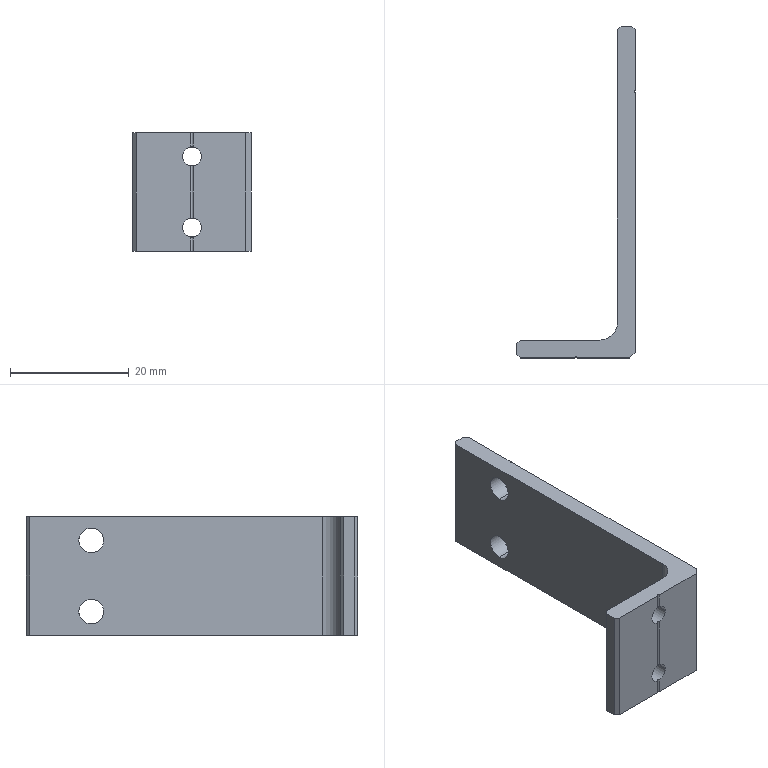Part | SolidWorks | features BaseBody 1 | 1 solid | 30 faces | box 20 x 56 x 20 mm | volume 4261 mm3 | cylinder 15 | plane 15 | commonest cylinder face diameters 0.4 x6 3.2 x4 4.2 x4 6 x1
STEP:
#1=CARTESIAN_POINT('',(20.,44.8,1.91));
#2=VERTEX_POINT('',#1);
#3=CARTESIAN_POINT('',(19.8,45.,1.9));
#4=VERTEX_POINT('',#3);
#5=CARTESIAN_POINT('',(20.,44.8,1.91));
#6=CARTESIAN_POINT('',(19.947,44.8,1.91));
#7=CARTESIAN_POINT('',(19.895,44.822,1.907));
#8=CARTESIAN_POINT('',(19.822,44.895,1.902));
#9=CARTESIAN_POINT('',(19.8,44.947,1.9));
#10=CARTESIAN_POINT('',(19.8,45.,1.9));
#11=B_SPLINE_CURVE_WITH_KNOTS('',3,(#5,#6,#7,#8,#9,#10),.UNSPECIFIED.,.F.,.F.,(4,2,4),(-0.0003126,-0.0001563,0.),.UNSPECIFIED.);
#12=EDGE_CURVE('',#2,#4,#11,.T.);
#13=ORIENTED_EDGE('',*,*,#12,.T.);
#14=CARTESIAN_POINT('',(17.,45.,1.9));
#15=VERTEX_POINT('',#14);
#16=CARTESIAN_POINT('',(37.,45.,1.9));
#17=DIRECTION('',(-1.,0.,0.));
#18=VECTOR('',#17,1000.);
#19=LINE('',#16,#18);
#20=EDGE_CURVE('',#4,#15,#19,.T.);
#21=ORIENTED_EDGE('',*,*,#20,.T.);
#22=CARTESIAN_POINT('',(17.,45.,6.1));
#23=VERTEX_POINT('',#22);
#24=CARTESIAN_POINT('',(17.,45.,4.));
#25=DIRECTION('',(-1.,0.,0.));
#26=DIRECTION('',(0.,0.,1.));
#27=AXIS2_PLACEMENT_3D('',#24,#25,#26);
#28=CIRCLE('',#27,2.1);
#29=EDGE_CURVE('',#15,#23,#28,.T.);
#30=ORIENTED_EDGE('',*,*,#29,.T.);
#31=CARTESIAN_POINT('',(19.8,45.,6.1));
#32=VERTEX_POINT('',#31);
#33=CARTESIAN_POINT('',(37.,45.,6.1));
#34=DIRECTION('',(-1.,0.,0.));
#35=VECTOR('',#34,1000.);
#36=LINE('',#33,#35);
#37=EDGE_CURVE('',#32,#23,#36,.T.);
#38=ORIENTED_EDGE('',*,*,#37,.F.);
#39=CARTESIAN_POINT('',(20.,44.8,6.09));
#40=VERTEX_POINT('',#39);
#41=CARTESIAN_POINT('',(19.8,45.,6.1));
#42=CARTESIAN_POINT('',(19.8,44.947,6.1));
#43=CARTESIAN_POINT('',(19.822,44.895,6.098));
#44=CARTESIAN_POINT('',(19.895,44.822,6.093));
#45=CARTESIAN_POINT('',(19.947,44.8,6.09));
#46=CARTESIAN_POINT('',(20.,44.8,6.09));
#47=B_SPLINE_CURVE_WITH_KNOTS('',3,(#41,#42,#43,#44,#45,#46),.UNSPECIFIED.,.F.,.F.,(4,2,4),(0.,0.0001563,0.0003126),.UNSPECIFIED.);
#48=EDGE_CURVE('',#32,#40,#47,.T.);
#49=ORIENTED_EDGE('',*,*,#48,.T.);
#50=CARTESIAN_POINT('',(20.,45.,4.));
#51=DIRECTION('',(-1.,0.,0.));
#52=DIRECTION('',(0.,0.,1.));
#53=AXIS2_PLACEMENT_3D('',#50,#51,#52);
#54=CIRCLE('',#53,2.1);
#55=EDGE_CURVE('',#2,#40,#54,.T.);
#56=ORIENTED_EDGE('',*,*,#55,.F.);
#57=EDGE_LOOP('',(#13,#21,#30,#38,#49,#56));
#58=FACE_OUTER_BOUND('',#57,.T.);
#59=CARTESIAN_POINT('',(37.,45.,4.));
#60=DIRECTION('',(-1.,0.,0.));
#61=DIRECTION('',(0.,0.,1.));
#62=AXIS2_PLACEMENT_3D('',#59,#60,#61);
#63=CYLINDRICAL_SURFACE('',#62,2.1);
#64=ADVANCED_FACE('',(#58),#63,.F.);
#65=CARTESIAN_POINT('',(20.,44.8,13.91));
#66=VERTEX_POINT('',#65);
#67=CARTESIAN_POINT('',(19.8,45.,13.9));
#68=VERTEX_POINT('',#67);
#69=CARTESIAN_POINT('',(20.,44.8,13.91));
#70=CARTESIAN_POINT('',(19.947,44.8,13.91));
#71=CARTESIAN_POINT('',(19.895,44.822,13.907));
#72=CARTESIAN_POINT('',(19.822,44.895,13.902));
#73=CARTESIAN_POINT('',(19.8,44.947,13.9));
#74=CARTESIAN_POINT('',(19.8,45.,13.9));
#75=B_SPLINE_CURVE_WITH_KNOTS('',3,(#69,#70,#71,#72,#73,#74),.UNSPECIFIED.,.F.,.F.,(4,2,4),(-0.0003126,-0.0001563,0.),.UNSPECIFIED.);
#76=EDGE_CURVE('',#66,#68,#75,.T.);
#77=ORIENTED_EDGE('',*,*,#76,.T.);
#78=CARTESIAN_POINT('',(17.,45.,13.9));
#79=VERTEX_POINT('',#78);
#80=CARTESIAN_POINT('',(37.,45.,13.9));
#81=DIRECTION('',(-1.,0.,0.));
#82=VECTOR('',#81,1000.);
#83=LINE('',#80,#82);
#84=EDGE_CURVE('',#68,#79,#83,.T.);
#85=ORIENTED_EDGE('',*,*,#84,.T.);
#86=CARTESIAN_POINT('',(17.,45.,18.1));
#87=VERTEX_POINT('',#86);
#88=CARTESIAN_POINT('',(17.,45.,16.));
#89=DIRECTION('',(-1.,0.,0.));
#90=DIRECTION('',(0.,0.,1.));
#91=AXIS2_PLACEMENT_3D('',#88,#89,#90);
#92=CIRCLE('',#91,2.1);
#93=EDGE_CURVE('',#79,#87,#92,.T.);
#94=ORIENTED_EDGE('',*,*,#93,.T.);
#95=CARTESIAN_POINT('',(19.8,45.,18.1));
#96=VERTEX_POINT('',#95);
#97=CARTESIAN_POINT('',(37.,45.,18.1));
#98=DIRECTION('',(-1.,0.,0.));
#99=VECTOR('',#98,1000.);
#100=LINE('',#97,#99);
#101=EDGE_CURVE('',#96,#87,#100,.T.);
#102=ORIENTED_EDGE('',*,*,#101,.F.);
#103=CARTESIAN_POINT('',(20.,44.8,18.09));
#104=VERTEX_POINT('',#103);
#105=CARTESIAN_POINT('',(19.8,45.,18.1));
#106=CARTESIAN_POINT('',(19.8,44.947,18.1));
#107=CARTESIAN_POINT('',(19.822,44.895,18.098));
#108=CARTESIAN_POINT('',(19.895,44.822,18.093));
#109=CARTESIAN_POINT('',(19.947,44.8,18.09));
#110=CARTESIAN_POINT('',(20.,44.8,18.09));
#111=B_SPLINE_CURVE_WITH_KNOTS('',3,(#105,#106,#107,#108,#109,#110),.UNSPECIFIED.,.F.,.F.,(4,2,4),(0.0003126,0.0004689,0.0006252),.UNSPECIFIED.);
#112=EDGE_CURVE('',#96,#104,#111,.T.);
#113=ORIENTED_EDGE('',*,*,#112,.T.);
#114=CARTESIAN_POINT('',(20.,45.,16.));
#115=DIRECTION('',(-1.,0.,0.));
#116=DIRECTION('',(0.,0.,1.));
#117=AXIS2_PLACEMENT_3D('',#114,#115,#116);
#118=CIRCLE('',#117,2.1);
#119=EDGE_CURVE('',#66,#104,#118,.T.);
#120=ORIENTED_EDGE('',*,*,#119,.F.);
#121=EDGE_LOOP('',(#77,#85,#94,#102,#113,#120));
#122=FACE_OUTER_BOUND('',#121,.T.);
#123=CARTESIAN_POINT('',(37.,45.,16.));
#124=DIRECTION('',(-1.,0.,0.));
#125=DIRECTION('',(0.,0.,1.));
#126=AXIS2_PLACEMENT_3D('',#123,#124,#125);
#127=CYLINDRICAL_SURFACE('',#126,2.1);
#128=ADVANCED_FACE('',(#122),#127,.F.);
#129=CARTESIAN_POINT('',(10.2,0.,2.413));
#130=VERTEX_POINT('',#129);
#131=CARTESIAN_POINT('',(11.6,0.,4.));
#132=VERTEX_POINT('',#131);
#133=CARTESIAN_POINT('',(10.,0.,4.));
#134=DIRECTION('',(0.,-1.,0.));
#135=DIRECTION('',(-1.,0.,0.));
#136=AXIS2_PLACEMENT_3D('',#133,#134,#135);
#137=CIRCLE('',#136,1.6);
#138=EDGE_CURVE('',#130,#132,#137,.T.);
#139=ORIENTED_EDGE('',*,*,#138,.T.);
#140=CARTESIAN_POINT('',(11.6,3.,4.));
#141=VERTEX_POINT('',#140);
#142=CARTESIAN_POINT('',(11.6,-17.,4.));
#143=DIRECTION('',(0.,1.,0.));
#144=VECTOR('',#143,1000.);
#145=LINE('',#142,#144);
#146=EDGE_CURVE('',#132,#141,#145,.T.);
#147=ORIENTED_EDGE('',*,*,#146,.T.);
#148=CARTESIAN_POINT('',(8.4,3.,4.));
#149=VERTEX_POINT('',#148);
#150=CARTESIAN_POINT('',(10.,3.,4.));
#151=DIRECTION('',(0.,1.,0.));
#152=DIRECTION('',(-1.,0.,0.));
#153=AXIS2_PLACEMENT_3D('',#150,#151,#152);
#154=CIRCLE('',#153,1.6);
#155=EDGE_CURVE('',#141,#149,#154,.T.);
#156=ORIENTED_EDGE('',*,*,#155,.T.);
#157=CARTESIAN_POINT('',(8.4,0.,4.));
#158=VERTEX_POINT('',#157);
#159=CARTESIAN_POINT('',(8.4,-17.,4.));
#160=DIRECTION('',(0.,1.,0.));
#161=VECTOR('',#160,1000.);
#162=LINE('',#159,#161);
#163=EDGE_CURVE('',#158,#149,#162,.T.);
#164=ORIENTED_EDGE('',*,*,#163,.F.);
#165=CARTESIAN_POINT('',(9.8,0.,2.413));
#166=VERTEX_POINT('',#165);
#167=CARTESIAN_POINT('',(10.,0.,4.));
#168=DIRECTION('',(0.,-1.,0.));
#169=DIRECTION('',(-1.,0.,0.));
#170=AXIS2_PLACEMENT_3D('',#167,#168,#169);
#171=CIRCLE('',#170,1.6);
#172=EDGE_CURVE('',#158,#166,#171,.T.);
#173=ORIENTED_EDGE('',*,*,#172,.T.);
#174=CARTESIAN_POINT('',(9.8,0.,2.413));
#175=CARTESIAN_POINT('',(9.8,0.0529,2.413));
#176=CARTESIAN_POINT('',(9.822,0.1046,2.41));
#177=CARTESIAN_POINT('',(9.895,0.1783,2.403));
#178=CARTESIAN_POINT('',(9.948,0.2,2.4));
#179=CARTESIAN_POINT('',(10.052,0.2,2.4));
#180=CARTESIAN_POINT('',(10.104,0.1788,2.403));
#181=CARTESIAN_POINT('',(10.179,0.1042,2.41));
#182=CARTESIAN_POINT('',(10.2,0.0529,2.413));
#183=CARTESIAN_POINT('',(10.2,0.,2.413));
#184=B_SPLINE_CURVE_WITH_KNOTS('',3,(#174,#175,#176,#177,#178,#179,#180,#181,#182,#183),.UNSPECIFIED.,.F.,.F.,(4,2,2,2,4),(0.,0.0001564,0.0003129,0.0004693,0.0006258),.UNSPECIFIED.);
#185=EDGE_CURVE('',#166,#130,#184,.T.);
#186=ORIENTED_EDGE('',*,*,#185,.T.);
#187=EDGE_LOOP('',(#139,#147,#156,#164,#173,#186));
#188=FACE_OUTER_BOUND('',#187,.T.);
#189=CARTESIAN_POINT('',(10.,-17.,4.));
#190=DIRECTION('',(0.,1.,0.));
#191=DIRECTION('',(-1.,0.,0.));
#192=AXIS2_PLACEMENT_3D('',#189,#190,#191);
#193=CYLINDRICAL_SURFACE('',#192,1.6);
#194=ADVANCED_FACE('',(#188),#193,.F.);
#195=CARTESIAN_POINT('',(10.2,0.,14.413));
#196=VERTEX_POINT('',#195);
#197=CARTESIAN_POINT('',(11.6,0.,16.));
#198=VERTEX_POINT('',#197);
#199=CARTESIAN_POINT('',(10.,0.,16.));
#200=DIRECTION('',(0.,-1.,0.));
#201=DIRECTION('',(-1.,0.,0.));
#202=AXIS2_PLACEMENT_3D('',#199,#200,#201);
#203=CIRCLE('',#202,1.6);
#204=EDGE_CURVE('',#196,#198,#203,.T.);
#205=ORIENTED_EDGE('',*,*,#204,.T.);
#206=CARTESIAN_POINT('',(11.6,3.,16.));
#207=VERTEX_POINT('',#206);
#208=CARTESIAN_POINT('',(11.6,-17.,16.));
#209=DIRECTION('',(0.,1.,0.));
#210=VECTOR('',#209,1000.);
#211=LINE('',#208,#210);
#212=EDGE_CURVE('',#198,#207,#211,.T.);
#213=ORIENTED_EDGE('',*,*,#212,.T.);
#214=CARTESIAN_POINT('',(8.4,3.,16.));
#215=VERTEX_POINT('',#214);
#216=CARTESIAN_POINT('',(10.,3.,16.));
#217=DIRECTION('',(0.,1.,0.));
#218=DIRECTION('',(-1.,0.,0.));
#219=AXIS2_PLACEMENT_3D('',#216,#217,#218);
#220=CIRCLE('',#219,1.6);
#221=EDGE_CURVE('',#207,#215,#220,.T.);
#222=ORIENTED_EDGE('',*,*,#221,.T.);
#223=CARTESIAN_POINT('',(8.4,0.,16.));
#224=VERTEX_POINT('',#223);
#225=CARTESIAN_POINT('',(8.4,-17.,16.));
#226=DIRECTION('',(0.,1.,0.));
#227=VECTOR('',#226,1000.);
#228=LINE('',#225,#227);
#229=EDGE_CURVE('',#224,#215,#228,.T.);
#230=ORIENTED_EDGE('',*,*,#229,.F.);
#231=CARTESIAN_POINT('',(9.8,0.,14.413));
#232=VERTEX_POINT('',#231);
#233=CARTESIAN_POINT('',(10.,0.,16.));
#234=DIRECTION('',(0.,-1.,0.));
#235=DIRECTION('',(-1.,0.,0.));
#236=AXIS2_PLACEMENT_3D('',#233,#234,#235);
#237=CIRCLE('',#236,1.6);
#238=EDGE_CURVE('',#224,#232,#237,.T.);
#239=ORIENTED_EDGE('',*,*,#238,.T.);
#240=CARTESIAN_POINT('',(9.8,0.,14.413));
#241=CARTESIAN_POINT('',(9.8,0.0529,14.413));
#242=CARTESIAN_POINT('',(9.822,0.1046,14.41));
#243=CARTESIAN_POINT('',(9.895,0.1783,14.403));
#244=CARTESIAN_POINT('',(9.948,0.2,14.4));
#245=CARTESIAN_POINT('',(10.052,0.2,14.4));
#246=CARTESIAN_POINT('',(10.104,0.1788,14.403));
#247=CARTESIAN_POINT('',(10.179,0.1042,14.41));
#248=CARTESIAN_POINT('',(10.2,0.0529,14.413));
#249=CARTESIAN_POINT('',(10.2,0.,14.413));
#250=B_SPLINE_CURVE_WITH_KNOTS('',3,(#240,#241,#242,#243,#244,#245,#246,#247,#248,#249),.UNSPECIFIED.,.F.,.F.,(4,2,2,2,4),(0.,0.0001564,0.0003129,0.0004693,0.0006258),.UNSPECIFIED.);
#251=EDGE_CURVE('',#232,#196,#250,.T.);
#252=ORIENTED_EDGE('',*,*,#251,.T.);
#253=EDGE_LOOP('',(#205,#213,#222,#230,#239,#252));
#254=FACE_OUTER_BOUND('',#253,.T.);
#255=CARTESIAN_POINT('',(10.,-17.,16.));
#256=DIRECTION('',(0.,1.,0.));
#257=DIRECTION('',(-1.,0.,0.));
#258=AXIS2_PLACEMENT_3D('',#255,#256,#257);
#259=CYLINDRICAL_SURFACE('',#258,1.6);
#260=ADVANCED_FACE('',(#254),#259,.F.);
#261=CARTESIAN_POINT('',(17.,55.4,0.));
#262=VERTEX_POINT('',#261);
#263=CARTESIAN_POINT('',(17.,55.4,20.));
#264=VERTEX_POINT('',#263);
#265=CARTESIAN_POINT('',(17.,55.4,20.));
#266=DIRECTION('',(0.,0.,1.));
#267=VECTOR('',#266,1000.);
#268=LINE('',#265,#267);
#269=EDGE_CURVE('',#262,#264,#268,.T.);
#270=ORIENTED_EDGE('',*,*,#269,.F.);
#271=CARTESIAN_POINT('',(17.,6.,0.));
#272=VERTEX_POINT('',#271);
#273=CARTESIAN_POINT('',(17.,56.,0.));
#274=DIRECTION('',(0.,1.,0.));
#275=VECTOR('',#274,1000.);
#276=LINE('',#273,#275);
#277=EDGE_CURVE('',#272,#262,#276,.T.);
#278=ORIENTED_EDGE('',*,*,#277,.F.);
#279=CARTESIAN_POINT('',(17.,6.,20.));
#280=VERTEX_POINT('',#279);
#281=CARTESIAN_POINT('',(17.,6.,20.));
#282=DIRECTION('',(0.,0.,-1.));
#283=VECTOR('',#282,1000.);
#284=LINE('',#281,#283);
#285=EDGE_CURVE('',#280,#272,#284,.T.);
#286=ORIENTED_EDGE('',*,*,#285,.F.);
#287=CARTESIAN_POINT('',(17.,56.,20.));
#288=DIRECTION('',(0.,-1.,0.));
#289=VECTOR('',#288,1000.);
#290=LINE('',#287,#289);
#291=EDGE_CURVE('',#264,#280,#290,.T.);
#292=ORIENTED_EDGE('',*,*,#291,.F.);
#293=EDGE_LOOP('',(#270,#278,#286,#292));
#294=FACE_OUTER_BOUND('',#293,.T.);
#295=CARTESIAN_POINT('',(17.,45.,4.));
#296=DIRECTION('',(-1.,0.,0.));
#297=DIRECTION('',(0.,0.,1.));
#298=AXIS2_PLACEMENT_3D('',#295,#296,#297);
#299=CIRCLE('',#298,2.1);
#300=EDGE_CURVE('',#23,#15,#299,.T.);
#301=ORIENTED_EDGE('',*,*,#300,.F.);
#302=ORIENTED_EDGE('',*,*,#29,.F.);
#303=EDGE_LOOP('',(#301,#302));
#304=FACE_BOUND('',#303,.T.);
#305=CARTESIAN_POINT('',(17.,45.,16.));
#306=DIRECTION('',(-1.,0.,0.));
#307=DIRECTION('',(0.,0.,1.));
#308=AXIS2_PLACEMENT_3D('',#305,#306,#307);
#309=CIRCLE('',#308,2.1);
#310=EDGE_CURVE('',#87,#79,#309,.T.);
#311=ORIENTED_EDGE('',*,*,#310,.F.);
#312=ORIENTED_EDGE('',*,*,#93,.F.);
#313=EDGE_LOOP('',(#311,#312));
#314=FACE_BOUND('',#313,.T.);
#315=CARTESIAN_POINT('',(17.,56.,20.));
#316=DIRECTION('',(1.,0.,0.));
#317=DIRECTION('',(0.,0.,-1.));
#318=AXIS2_PLACEMENT_3D('',#315,#316,#317);
#319=PLANE('',#318);
#320=ADVANCED_FACE('',(#294,#304,#314),#319,.F.);
#321=CARTESIAN_POINT('',(0.,0.6,20.));
#322=VERTEX_POINT('',#321);
#323=CARTESIAN_POINT('',(0.6,0.,20.));
#324=VERTEX_POINT('',#323);
#325=CARTESIAN_POINT('',(0.6,0.,20.));
#326=DIRECTION('',(0.7071,-0.7071,0.));
#327=VECTOR('',#326,1000.);
#328=LINE('',#325,#327);
#329=EDGE_CURVE('',#322,#324,#328,.T.);
#330=ORIENTED_EDGE('',*,*,#329,.T.);
#331=CARTESIAN_POINT('',(9.8,0.,20.));
#332=VERTEX_POINT('',#331);
#333=CARTESIAN_POINT('',(0.,0.,20.));
#334=DIRECTION('',(1.,0.,0.));
#335=VECTOR('',#334,1000.);
#336=LINE('',#333,#335);
#337=EDGE_CURVE('',#324,#332,#336,.T.);
#338=ORIENTED_EDGE('',*,*,#337,.T.);
#339=CARTESIAN_POINT('',(10.2,0.,20.));
#340=VERTEX_POINT('',#339);
#341=CARTESIAN_POINT('',(10.,0.,20.));
#342=DIRECTION('',(0.,0.,-1.));
#343=DIRECTION('',(1.,0.,0.));
#344=AXIS2_PLACEMENT_3D('',#341,#342,#343);
#345=CIRCLE('',#344,0.2);
#346=EDGE_CURVE('',#332,#340,#345,.T.);
#347=ORIENTED_EDGE('',*,*,#346,.T.);
#348=CARTESIAN_POINT('',(19.,0.,20.));
#349=VERTEX_POINT('',#348);
#350=CARTESIAN_POINT('',(0.,0.,20.));
#351=DIRECTION('',(1.,0.,0.));
#352=VECTOR('',#351,1000.);
#353=LINE('',#350,#352);
#354=EDGE_CURVE('',#340,#349,#353,.T.);
#355=ORIENTED_EDGE('',*,*,#354,.T.);
#356=CARTESIAN_POINT('',(20.,1.,20.));
#357=VERTEX_POINT('',#356);
#358=CARTESIAN_POINT('',(20.,1.,20.));
#359=DIRECTION('',(0.7071,0.7071,0.));
#360=VECTOR('',#359,1000.);
#361=LINE('',#358,#360);
#362=EDGE_CURVE('',#349,#357,#361,.T.);
#363=ORIENTED_EDGE('',*,*,#362,.T.);
#364=CARTESIAN_POINT('',(20.,44.8,20.));
#365=VERTEX_POINT('',#364);
#366=CARTESIAN_POINT('',(20.,0.,20.));
#367=DIRECTION('',(0.,1.,0.));
#368=VECTOR('',#367,1000.);
#369=LINE('',#366,#368);
#370=EDGE_CURVE('',#357,#365,#369,.T.);
#371=ORIENTED_EDGE('',*,*,#370,.T.);
#372=CARTESIAN_POINT('',(20.,45.2,20.));
#373=VERTEX_POINT('',#372);
#374=CARTESIAN_POINT('',(20.,45.,20.));
#375=DIRECTION('',(0.,0.,-1.));
#376=DIRECTION('',(1.,0.,0.));
#377=AXIS2_PLACEMENT_3D('',#374,#375,#376);
#378=CIRCLE('',#377,0.2);
#379=EDGE_CURVE('',#365,#373,#378,.T.);
#380=ORIENTED_EDGE('',*,*,#379,.T.);
#381=CARTESIAN_POINT('',(20.,55.4,20.));
#382=VERTEX_POINT('',#381);
#383=CARTESIAN_POINT('',(20.,0.,20.));
#384=DIRECTION('',(0.,1.,0.));
#385=VECTOR('',#384,1000.);
#386=LINE('',#383,#385);
#387=EDGE_CURVE('',#373,#382,#386,.T.);
#388=ORIENTED_EDGE('',*,*,#387,.T.);
#389=CARTESIAN_POINT('',(19.4,56.,20.));
#390=VERTEX_POINT('',#389);
#391=CARTESIAN_POINT('',(19.4,56.,20.));
#392=DIRECTION('',(-0.7071,0.7071,0.));
#393=VECTOR('',#392,1000.);
#394=LINE('',#391,#393);
#395=EDGE_CURVE('',#382,#390,#394,.T.);
#396=ORIENTED_EDGE('',*,*,#395,.T.);
#397=CARTESIAN_POINT('',(17.6,56.,20.));
#398=VERTEX_POINT('',#397);
#399=CARTESIAN_POINT('',(0.,56.,20.));
#400=DIRECTION('',(-1.,0.,0.));
#401=VECTOR('',#400,1000.);
#402=LINE('',#399,#401);
#403=EDGE_CURVE('',#390,#398,#402,.T.);
#404=ORIENTED_EDGE('',*,*,#403,.T.);
#405=CARTESIAN_POINT('',(17.6,56.,20.));
#406=DIRECTION('',(-0.7071,-0.7071,0.));
#407=VECTOR('',#406,1000.);
#408=LINE('',#405,#407);
#409=EDGE_CURVE('',#398,#264,#408,.T.);
#410=ORIENTED_EDGE('',*,*,#409,.T.);
#411=ORIENTED_EDGE('',*,*,#291,.T.);
#412=CARTESIAN_POINT('',(14.,3.,20.));
#413=VERTEX_POINT('',#412);
#414=CARTESIAN_POINT('',(14.,6.,20.));
#415=DIRECTION('',(0.,0.,-1.));
#416=DIRECTION('',(1.,0.,0.));
#417=AXIS2_PLACEMENT_3D('',#414,#415,#416);
#418=CIRCLE('',#417,3.);
#419=EDGE_CURVE('',#280,#413,#418,.T.);
#420=ORIENTED_EDGE('',*,*,#419,.T.);
#421=CARTESIAN_POINT('',(0.6,3.,20.));
#422=VERTEX_POINT('',#421);
#423=CARTESIAN_POINT('',(0.,3.,20.));
#424=DIRECTION('',(-1.,0.,0.));
#425=VECTOR('',#424,1000.);
#426=LINE('',#423,#425);
#427=EDGE_CURVE('',#413,#422,#426,.T.);
#428=ORIENTED_EDGE('',*,*,#427,.T.);
#429=CARTESIAN_POINT('',(0.,2.4,20.));
#430=VERTEX_POINT('',#429);
#431=CARTESIAN_POINT('',(0.,2.4,20.));
#432=DIRECTION('',(-0.7071,-0.7071,0.));
#433=VECTOR('',#432,1000.);
#434=LINE('',#431,#433);
#435=EDGE_CURVE('',#422,#430,#434,.T.);
#436=ORIENTED_EDGE('',*,*,#435,.T.);
#437=CARTESIAN_POINT('',(0.,0.,20.));
#438=DIRECTION('',(0.,-1.,0.));
#439=VECTOR('',#438,1000.);
#440=LINE('',#437,#439);
#441=EDGE_CURVE('',#430,#322,#440,.T.);
#442=ORIENTED_EDGE('',*,*,#441,.T.);
#443=EDGE_LOOP('',(#330,#338,#347,#355,#363,#371,#380,#388,#396,#404,#410,#411,#420,#428,#436,#442));
#444=FACE_OUTER_BOUND('',#443,.T.);
#445=CARTESIAN_POINT('',(0.,0.,20.));
#446=DIRECTION('',(0.,0.,1.));
#447=DIRECTION('',(1.,0.,0.));
#448=AXIS2_PLACEMENT_3D('',#445,#446,#447);
#449=PLANE('',#448);
#450=ADVANCED_FACE('',(#444),#449,.T.);
#451=CARTESIAN_POINT('',(17.6,56.,0.));
#452=VERTEX_POINT('',#451);
#453=CARTESIAN_POINT('',(17.6,56.,20.));
#454=DIRECTION('',(0.,0.,1.));
#455=VECTOR('',#454,1000.);
#456=LINE('',#453,#455);
#457=EDGE_CURVE('',#452,#398,#456,.T.);
#458=ORIENTED_EDGE('',*,*,#457,.F.);
#459=CARTESIAN_POINT('',(17.,55.4,0.));
#460=DIRECTION('',(0.7071,0.7071,0.));
#461=VECTOR('',#460,1000.);
#462=LINE('',#459,#461);
#463=EDGE_CURVE('',#262,#452,#462,.T.);
#464=ORIENTED_EDGE('',*,*,#463,.F.);
#465=ORIENTED_EDGE('',*,*,#269,.T.);
#466=ORIENTED_EDGE('',*,*,#409,.F.);
#467=EDGE_LOOP('',(#458,#464,#465,#466));
#468=FACE_OUTER_BOUND('',#467,.T.);
#469=CARTESIAN_POINT('',(17.,55.4,20.));
#470=DIRECTION('',(0.7071,-0.7071,0.));
#471=DIRECTION('',(0.7071,0.7071,0.));
#472=AXIS2_PLACEMENT_3D('',#469,#470,#471);
#473=PLANE('',#472);
#474=ADVANCED_FACE('',(#468),#473,.F.);
#475=CARTESIAN_POINT('',(10.2,0.,0.));
#476=VERTEX_POINT('',#475);
#477=CARTESIAN_POINT('',(9.8,0.,0.));
#478=VERTEX_POINT('',#477);
#479=CARTESIAN_POINT('',(10.,0.,0.));
#480=DIRECTION('',(0.,0.,1.));
#481=DIRECTION('',(1.,0.,0.));
#482=AXIS2_PLACEMENT_3D('',#479,#480,#481);
#483=CIRCLE('',#482,0.2);
#484=EDGE_CURVE('',#476,#478,#483,.T.);
#485=ORIENTED_EDGE('',*,*,#484,.T.);
#486=CARTESIAN_POINT('',(0.6,0.,0.));
#487=VERTEX_POINT('',#486);
#488=CARTESIAN_POINT('',(0.,0.,0.));
#489=DIRECTION('',(1.,0.,0.));
#490=VECTOR('',#489,1000.);
#491=LINE('',#488,#490);
#492=EDGE_CURVE('',#487,#478,#491,.T.);
#493=ORIENTED_EDGE('',*,*,#492,.F.);
#494=CARTESIAN_POINT('',(0.,0.6,0.));
#495=VERTEX_POINT('',#494);
#496=CARTESIAN_POINT('',(0.6,0.,0.));
#497=DIRECTION('',(-0.7071,0.7071,0.));
#498=VECTOR('',#497,1000.);
#499=LINE('',#496,#498);
#500=EDGE_CURVE('',#487,#495,#499,.T.);
#501=ORIENTED_EDGE('',*,*,#500,.T.);
#502=CARTESIAN_POINT('',(0.,2.4,0.));
#503=VERTEX_POINT('',#502);
#504=CARTESIAN_POINT('',(0.,0.,0.));
#505=DIRECTION('',(0.,-1.,0.));
#506=VECTOR('',#505,1000.);
#507=LINE('',#504,#506);
#508=EDGE_CURVE('',#503,#495,#507,.T.);
#509=ORIENTED_EDGE('',*,*,#508,.F.);
#510=CARTESIAN_POINT('',(0.6,3.,0.));
#511=VERTEX_POINT('',#510);
#512=CARTESIAN_POINT('',(0.,2.4,0.));
#513=DIRECTION('',(0.7071,0.7071,0.));
#514=VECTOR('',#513,1000.);
#515=LINE('',#512,#514);
#516=EDGE_CURVE('',#503,#511,#515,.T.);
#517=ORIENTED_EDGE('',*,*,#516,.T.);
#518=CARTESIAN_POINT('',(14.,3.,0.));
#519=VERTEX_POINT('',#518);
#520=CARTESIAN_POINT('',(0.,3.,0.));
#521=DIRECTION('',(-1.,0.,0.));
#522=VECTOR('',#521,1000.);
#523=LINE('',#520,#522);
#524=EDGE_CURVE('',#519,#511,#523,.T.);
#525=ORIENTED_EDGE('',*,*,#524,.F.);
#526=CARTESIAN_POINT('',(14.,6.,0.));
#527=DIRECTION('',(0.,0.,-1.));
#528=DIRECTION('',(1.,0.,0.));
#529=AXIS2_PLACEMENT_3D('',#526,#527,#528);
#530=CIRCLE('',#529,3.);
#531=EDGE_CURVE('',#272,#519,#530,.T.);
#532=ORIENTED_EDGE('',*,*,#531,.F.);
#533=ORIENTED_EDGE('',*,*,#277,.T.);
#534=ORIENTED_EDGE('',*,*,#463,.T.);
#535=CARTESIAN_POINT('',(19.4,56.,0.));
#536=VERTEX_POINT('',#535);
#537=CARTESIAN_POINT('',(0.,56.,0.));
#538=DIRECTION('',(-1.,0.,0.));
#539=VECTOR('',#538,1000.);
#540=LINE('',#537,#539);
#541=EDGE_CURVE('',#536,#452,#540,.T.);
#542=ORIENTED_EDGE('',*,*,#541,.F.);
#543=CARTESIAN_POINT('',(20.,55.4,0.));
#544=VERTEX_POINT('',#543);
#545=CARTESIAN_POINT('',(19.4,56.,0.));
#546=DIRECTION('',(0.7071,-0.7071,0.));
#547=VECTOR('',#546,1000.);
#548=LINE('',#545,#547);
#549=EDGE_CURVE('',#536,#544,#548,.T.);
#550=ORIENTED_EDGE('',*,*,#549,.T.);
#551=CARTESIAN_POINT('',(20.,45.2,0.));
#552=VERTEX_POINT('',#551);
#553=CARTESIAN_POINT('',(20.,0.,0.));
#554=DIRECTION('',(0.,1.,0.));
#555=VECTOR('',#554,1000.);
#556=LINE('',#553,#555);
#557=EDGE_CURVE('',#552,#544,#556,.T.);
#558=ORIENTED_EDGE('',*,*,#557,.F.);
#559=CARTESIAN_POINT('',(20.,44.8,0.));
#560=VERTEX_POINT('',#559);
#561=CARTESIAN_POINT('',(20.,45.,0.));
#562=DIRECTION('',(0.,0.,1.));
#563=DIRECTION('',(1.,0.,0.));
#564=AXIS2_PLACEMENT_3D('',#561,#562,#563);
#565=CIRCLE('',#564,0.2);
#566=EDGE_CURVE('',#552,#560,#565,.T.);
#567=ORIENTED_EDGE('',*,*,#566,.T.);
#568=CARTESIAN_POINT('',(20.,1.,0.));
#569=VERTEX_POINT('',#568);
#570=CARTESIAN_POINT('',(20.,0.,0.));
#571=DIRECTION('',(0.,1.,0.));
#572=VECTOR('',#571,1000.);
#573=LINE('',#570,#572);
#574=EDGE_CURVE('',#569,#560,#573,.T.);
#575=ORIENTED_EDGE('',*,*,#574,.F.);
#576=CARTESIAN_POINT('',(19.,0.,0.));
#577=VERTEX_POINT('',#576);
#578=CARTESIAN_POINT('',(20.,1.,0.));
#579=DIRECTION('',(-0.7071,-0.7071,0.));
#580=VECTOR('',#579,1000.);
#581=LINE('',#578,#580);
#582=EDGE_CURVE('',#569,#577,#581,.T.);
#583=ORIENTED_EDGE('',*,*,#582,.T.);
#584=CARTESIAN_POINT('',(0.,0.,0.));
#585=DIRECTION('',(1.,0.,0.));
#586=VECTOR('',#585,1000.);
#587=LINE('',#584,#586);
#588=EDGE_CURVE('',#476,#577,#587,.T.);
#589=ORIENTED_EDGE('',*,*,#588,.F.);
#590=EDGE_LOOP('',(#485,#493,#501,#509,#517,#525,#532,#533,#534,#542,#550,#558,#567,#575,#583,#589));
#591=FACE_OUTER_BOUND('',#590,.T.);
#592=CARTESIAN_POINT('',(0.,0.,0.));
#593=DIRECTION('',(0.,0.,1.));
#594=DIRECTION('',(1.,0.,0.));
#595=AXIS2_PLACEMENT_3D('',#592,#593,#594);
#596=PLANE('',#595);
#597=ADVANCED_FACE('',(#591),#596,.F.);
#598=ORIENTED_EDGE('',*,*,#285,.T.);
#599=ORIENTED_EDGE('',*,*,#531,.T.);
#600=CARTESIAN_POINT('',(14.,3.,20.));
#601=DIRECTION('',(0.,0.,-1.));
#602=VECTOR('',#601,1000.);
#603=LINE('',#600,#602);
#604=EDGE_CURVE('',#413,#519,#603,.T.);
#605=ORIENTED_EDGE('',*,*,#604,.F.);
#606=ORIENTED_EDGE('',*,*,#419,.F.);
#607=EDGE_LOOP('',(#598,#599,#605,#606));
#608=FACE_OUTER_BOUND('',#607,.T.);
#609=CARTESIAN_POINT('',(14.,6.,20.));
#610=DIRECTION('',(0.,0.,1.));
#611=DIRECTION('',(1.,0.,0.));
#612=AXIS2_PLACEMENT_3D('',#609,#610,#611);
#613=CYLINDRICAL_SURFACE('',#612,3.);
#614=ADVANCED_FACE('',(#608),#613,.F.);
#615=ORIENTED_EDGE('',*,*,#20,.F.);
#616=CARTESIAN_POINT('',(20.,45.2,1.91));
#617=VERTEX_POINT('',#616);
#618=CARTESIAN_POINT('',(19.8,45.,1.9));
#619=CARTESIAN_POINT('',(19.8,45.053,1.9));
#620=CARTESIAN_POINT('',(19.822,45.105,1.902));
#621=CARTESIAN_POINT('',(19.895,45.178,1.907));
#622=CARTESIAN_POINT('',(19.947,45.2,1.91));
#623=CARTESIAN_POINT('',(20.,45.2,1.91));
#624=B_SPLINE_CURVE_WITH_KNOTS('',3,(#618,#619,#620,#621,#622,#623),.UNSPECIFIED.,.F.,.F.,(4,2,4),(0.,0.0001563,0.0003126),.UNSPECIFIED.);
#625=EDGE_CURVE('',#4,#617,#624,.T.);
#626=ORIENTED_EDGE('',*,*,#625,.T.);
#627=CARTESIAN_POINT('',(20.,45.2,6.09));
#628=VERTEX_POINT('',#627);
#629=CARTESIAN_POINT('',(20.,45.,4.));
#630=DIRECTION('',(-1.,0.,0.));
#631=DIRECTION('',(0.,0.,1.));
#632=AXIS2_PLACEMENT_3D('',#629,#630,#631);
#633=CIRCLE('',#632,2.1);
#634=EDGE_CURVE('',#628,#617,#633,.T.);
#635=ORIENTED_EDGE('',*,*,#634,.F.);
#636=CARTESIAN_POINT('',(20.,45.2,6.09));
#637=CARTESIAN_POINT('',(19.947,45.2,6.09));
#638=CARTESIAN_POINT('',(19.895,45.178,6.093));
#639=CARTESIAN_POINT('',(19.822,45.105,6.098));
#640=CARTESIAN_POINT('',(19.8,45.053,6.1));
#641=CARTESIAN_POINT('',(19.8,45.,6.1));
#642=B_SPLINE_CURVE_WITH_KNOTS('',3,(#636,#637,#638,#639,#640,#641),.UNSPECIFIED.,.F.,.F.,(4,2,4),(-0.0003126,-0.0001563,0.),.UNSPECIFIED.);
#643=EDGE_CURVE('',#628,#32,#642,.T.);
#644=ORIENTED_EDGE('',*,*,#643,.T.);
#645=ORIENTED_EDGE('',*,*,#37,.T.);
#646=ORIENTED_EDGE('',*,*,#300,.T.);
#647=EDGE_LOOP('',(#615,#626,#635,#644,#645,#646));
#648=FACE_OUTER_BOUND('',#647,.T.);
#649=CARTESIAN_POINT('',(37.,45.,4.));
#650=DIRECTION('',(-1.,0.,0.));
#651=DIRECTION('',(0.,0.,1.));
#652=AXIS2_PLACEMENT_3D('',#649,#650,#651);
#653=CYLINDRICAL_SURFACE('',#652,2.1);
#654=ADVANCED_FACE('',(#648),#653,.F.);
#655=ORIENTED_EDGE('',*,*,#84,.F.);
#656=CARTESIAN_POINT('',(20.,45.2,13.91));
#657=VERTEX_POINT('',#656);
#658=CARTESIAN_POINT('',(19.8,45.,13.9));
#659=CARTESIAN_POINT('',(19.8,45.053,13.9));
#660=CARTESIAN_POINT('',(19.822,45.105,13.902));
#661=CARTESIAN_POINT('',(19.895,45.178,13.907));
#662=CARTESIAN_POINT('',(19.947,45.2,13.91));
#663=CARTESIAN_POINT('',(20.,45.2,13.91));
#664=B_SPLINE_CURVE_WITH_KNOTS('',3,(#658,#659,#660,#661,#662,#663),.UNSPECIFIED.,.F.,.F.,(4,2,4),(0.,0.0001563,0.0003126),.UNSPECIFIED.);
#665=EDGE_CURVE('',#68,#657,#664,.T.);
#666=ORIENTED_EDGE('',*,*,#665,.T.);
#667=CARTESIAN_POINT('',(20.,45.2,18.09));
#668=VERTEX_POINT('',#667);
#669=CARTESIAN_POINT('',(20.,45.,16.));
#670=DIRECTION('',(-1.,0.,0.));
#671=DIRECTION('',(0.,0.,1.));
#672=AXIS2_PLACEMENT_3D('',#669,#670,#671);
#673=CIRCLE('',#672,2.1);
#674=EDGE_CURVE('',#668,#657,#673,.T.);
#675=ORIENTED_EDGE('',*,*,#674,.F.);
#676=CARTESIAN_POINT('',(20.,45.2,18.09));
#677=CARTESIAN_POINT('',(19.947,45.2,18.09));
#678=CARTESIAN_POINT('',(19.895,45.178,18.093));
#679=CARTESIAN_POINT('',(19.822,45.105,18.098));
#680=CARTESIAN_POINT('',(19.8,45.053,18.1));
#681=CARTESIAN_POINT('',(19.8,45.,18.1));
#682=B_SPLINE_CURVE_WITH_KNOTS('',3,(#676,#677,#678,#679,#680,#681),.UNSPECIFIED.,.F.,.F.,(4,2,4),(0.,0.0001563,0.0003126),.UNSPECIFIED.);
#683=EDGE_CURVE('',#668,#96,#682,.T.);
#684=ORIENTED_EDGE('',*,*,#683,.T.);
#685=ORIENTED_EDGE('',*,*,#101,.T.);
#686=ORIENTED_EDGE('',*,*,#310,.T.);
#687=EDGE_LOOP('',(#655,#666,#675,#684,#685,#686));
#688=FACE_OUTER_BOUND('',#687,.T.);
#689=CARTESIAN_POINT('',(37.,45.,16.));
#690=DIRECTION('',(-1.,0.,0.));
#691=DIRECTION('',(0.,0.,1.));
#692=AXIS2_PLACEMENT_3D('',#689,#690,#691);
#693=CYLINDRICAL_SURFACE('',#692,2.1);
#694=ADVANCED_FACE('',(#688),#693,.F.);
#695=CARTESIAN_POINT('',(9.8,0.,20.));
#696=DIRECTION('',(0.,0.,-1.));
#697=VECTOR('',#696,1000.);
#698=LINE('',#695,#697);
#699=EDGE_CURVE('',#166,#478,#698,.T.);
#700=ORIENTED_EDGE('',*,*,#699,.F.);
#701=ORIENTED_EDGE('',*,*,#172,.F.);
#702=CARTESIAN_POINT('',(9.8,0.,5.587));
#703=VERTEX_POINT('',#702);
#704=CARTESIAN_POINT('',(10.,0.,4.));
#705=DIRECTION('',(0.,-1.,0.));
#706=DIRECTION('',(-1.,0.,0.));
#707=AXIS2_PLACEMENT_3D('',#704,#705,#706);
#708=CIRCLE('',#707,1.6);
#709=EDGE_CURVE('',#703,#158,#708,.T.);
#710=ORIENTED_EDGE('',*,*,#709,.F.);
#711=CARTESIAN_POINT('',(9.8,0.,20.));
#712=DIRECTION('',(0.,0.,-1.));
#713=VECTOR('',#712,1000.);
#714=LINE('',#711,#713);
#715=EDGE_CURVE('',#232,#703,#714,.T.);
#716=ORIENTED_EDGE('',*,*,#715,.F.);
#717=ORIENTED_EDGE('',*,*,#238,.F.);
#718=CARTESIAN_POINT('',(9.8,0.,17.587));
#719=VERTEX_POINT('',#718);
#720=CARTESIAN_POINT('',(10.,0.,16.));
#721=DIRECTION('',(0.,-1.,0.));
#722=DIRECTION('',(-1.,0.,0.));
#723=AXIS2_PLACEMENT_3D('',#720,#721,#722);
#724=CIRCLE('',#723,1.6);
#725=EDGE_CURVE('',#719,#224,#724,.T.);
#726=ORIENTED_EDGE('',*,*,#725,.F.);
#727=CARTESIAN_POINT('',(9.8,0.,20.));
#728=DIRECTION('',(0.,0.,-1.));
#729=VECTOR('',#728,1000.);
#730=LINE('',#727,#729);
#731=EDGE_CURVE('',#332,#719,#730,.T.);
#732=ORIENTED_EDGE('',*,*,#731,.F.);
#733=ORIENTED_EDGE('',*,*,#337,.F.);
#734=CARTESIAN_POINT('',(0.6,0.,20.));
#735=DIRECTION('',(0.,0.,1.));
#736=VECTOR('',#735,1000.);
#737=LINE('',#734,#736);
#738=EDGE_CURVE('',#487,#324,#737,.T.);
#739=ORIENTED_EDGE('',*,*,#738,.F.);
#740=ORIENTED_EDGE('',*,*,#492,.T.);
#741=EDGE_LOOP('',(#700,#701,#710,#716,#717,#726,#732,#733,#739,#740));
#742=FACE_OUTER_BOUND('',#741,.T.);
#743=CARTESIAN_POINT('',(0.,0.,20.));
#744=DIRECTION('',(0.,1.,0.));
#745=DIRECTION('',(0.,0.,1.));
#746=AXIS2_PLACEMENT_3D('',#743,#744,#745);
#747=PLANE('',#746);
#748=ADVANCED_FACE('',(#742),#747,.F.);
#749=CARTESIAN_POINT('',(0.,2.4,20.));
#750=DIRECTION('',(0.,0.,1.));
#751=VECTOR('',#750,1000.);
#752=LINE('',#749,#751);
#753=EDGE_CURVE('',#503,#430,#752,.T.);
#754=ORIENTED_EDGE('',*,*,#753,.F.);
#755=ORIENTED_EDGE('',*,*,#508,.T.);
#756=CARTESIAN_POINT('',(0.,0.6,20.));
#757=DIRECTION('',(0.,0.,-1.));
#758=VECTOR('',#757,1000.);
#759=LINE('',#756,#758);
#760=EDGE_CURVE('',#322,#495,#759,.T.);
#761=ORIENTED_EDGE('',*,*,#760,.F.);
#762=ORIENTED_EDGE('',*,*,#441,.F.);
#763=EDGE_LOOP('',(#754,#755,#761,#762));
#764=FACE_OUTER_BOUND('',#763,.T.);
#765=CARTESIAN_POINT('',(0.,3.,20.));
#766=DIRECTION('',(1.,0.,0.));
#767=DIRECTION('',(0.,1.,0.));
#768=AXIS2_PLACEMENT_3D('',#765,#766,#767);
#769=PLANE('',#768);
#770=ADVANCED_FACE('',(#764),#769,.F.);
#771=CARTESIAN_POINT('',(0.6,3.,20.));
#772=DIRECTION('',(0.,0.,-1.));
#773=VECTOR('',#772,1000.);
#774=LINE('',#771,#773);
#775=EDGE_CURVE('',#422,#511,#774,.T.);
#776=ORIENTED_EDGE('',*,*,#775,.F.);
#777=ORIENTED_EDGE('',*,*,#427,.F.);
#778=ORIENTED_EDGE('',*,*,#604,.T.);
#779=ORIENTED_EDGE('',*,*,#524,.T.);
#780=EDGE_LOOP('',(#776,#777,#778,#779));
#781=FACE_OUTER_BOUND('',#780,.T.);
#782=CARTESIAN_POINT('',(10.,3.,16.));
#783=DIRECTION('',(0.,1.,0.));
#784=DIRECTION('',(-1.,0.,0.));
#785=AXIS2_PLACEMENT_3D('',#782,#783,#784);
#786=CIRCLE('',#785,1.6);
#787=EDGE_CURVE('',#215,#207,#786,.T.);
#788=ORIENTED_EDGE('',*,*,#787,.F.);
#789=ORIENTED_EDGE('',*,*,#221,.F.);
#790=EDGE_LOOP('',(#788,#789));
#791=FACE_BOUND('',#790,.T.);
#792=CARTESIAN_POINT('',(10.,3.,4.));
#793=DIRECTION('',(0.,1.,0.));
#794=DIRECTION('',(-1.,0.,0.));
#795=AXIS2_PLACEMENT_3D('',#792,#793,#794);
#796=CIRCLE('',#795,1.6);
#797=EDGE_CURVE('',#149,#141,#796,.T.);
#798=ORIENTED_EDGE('',*,*,#797,.F.);
#799=ORIENTED_EDGE('',*,*,#155,.F.);
#800=EDGE_LOOP('',(#798,#799));
#801=FACE_BOUND('',#800,.T.);
#802=CARTESIAN_POINT('',(17.,3.,20.));
#803=DIRECTION('',(0.,-1.,0.));
#804=DIRECTION('',(1.,0.,0.));
#805=AXIS2_PLACEMENT_3D('',#802,#803,#804);
#806=PLANE('',#805);
#807=ADVANCED_FACE('',(#781,#791,#801),#806,.F.);
#808=CARTESIAN_POINT('',(19.4,56.,20.));
#809=DIRECTION('',(0.,0.,1.));
#810=VECTOR('',#809,1000.);
#811=LINE('',#808,#810);
#812=EDGE_CURVE('',#536,#390,#811,.T.);
#813=ORIENTED_EDGE('',*,*,#812,.F.);
#814=ORIENTED_EDGE('',*,*,#541,.T.);
#815=ORIENTED_EDGE('',*,*,#457,.T.);
#816=ORIENTED_EDGE('',*,*,#403,.F.);
#817=EDGE_LOOP('',(#813,#814,#815,#816));
#818=FACE_OUTER_BOUND('',#817,.T.);
#819=CARTESIAN_POINT('',(20.,56.,20.));
#820=DIRECTION('',(0.,-1.,0.));
#821=DIRECTION('',(0.,0.,-1.));
#822=AXIS2_PLACEMENT_3D('',#819,#820,#821);
#823=PLANE('',#822);
#824=ADVANCED_FACE('',(#818),#823,.F.);
#825=CARTESIAN_POINT('',(20.,45.2,20.));
#826=DIRECTION('',(0.,0.,1.));
#827=VECTOR('',#826,1000.);
#828=LINE('',#825,#827);
#829=EDGE_CURVE('',#668,#373,#828,.T.);
#830=ORIENTED_EDGE('',*,*,#829,.F.);
#831=ORIENTED_EDGE('',*,*,#674,.T.);
#832=CARTESIAN_POINT('',(20.,45.2,20.));
#833=DIRECTION('',(0.,0.,1.));
#834=VECTOR('',#833,1000.);
#835=LINE('',#832,#834);
#836=EDGE_CURVE('',#628,#657,#835,.T.);
#837=ORIENTED_EDGE('',*,*,#836,.F.);
#838=ORIENTED_EDGE('',*,*,#634,.T.);
#839=CARTESIAN_POINT('',(20.,45.2,20.));
#840=DIRECTION('',(0.,0.,1.));
#841=VECTOR('',#840,1000.);
#842=LINE('',#839,#841);
#843=EDGE_CURVE('',#552,#617,#842,.T.);
#844=ORIENTED_EDGE('',*,*,#843,.F.);
#845=ORIENTED_EDGE('',*,*,#557,.T.);
#846=CARTESIAN_POINT('',(20.,55.4,20.));
#847=DIRECTION('',(0.,0.,-1.));
#848=VECTOR('',#847,1000.);
#849=LINE('',#846,#848);
#850=EDGE_CURVE('',#382,#544,#849,.T.);
#851=ORIENTED_EDGE('',*,*,#850,.F.);
#852=ORIENTED_EDGE('',*,*,#387,.F.);
#853=EDGE_LOOP('',(#830,#831,#837,#838,#844,#845,#851,#852));
#854=FACE_OUTER_BOUND('',#853,.T.);
#855=CARTESIAN_POINT('',(20.,0.,20.));
#856=DIRECTION('',(-1.,0.,0.));
#857=DIRECTION('',(0.,0.,1.));
#858=AXIS2_PLACEMENT_3D('',#855,#856,#857);
#859=PLANE('',#858);
#860=ADVANCED_FACE('',(#854),#859,.F.);
#861=CARTESIAN_POINT('',(20.,44.8,20.));
#862=DIRECTION('',(0.,0.,-1.));
#863=VECTOR('',#862,1000.);
#864=LINE('',#861,#863);
#865=EDGE_CURVE('',#2,#560,#864,.T.);
#866=ORIENTED_EDGE('',*,*,#865,.F.);
#867=ORIENTED_EDGE('',*,*,#55,.T.);
#868=CARTESIAN_POINT('',(20.,44.8,20.));
#869=DIRECTION('',(0.,0.,-1.));
#870=VECTOR('',#869,1000.);
#871=LINE('',#868,#870);
#872=EDGE_CURVE('',#66,#40,#871,.T.);
#873=ORIENTED_EDGE('',*,*,#872,.F.);
#874=ORIENTED_EDGE('',*,*,#119,.T.);
#875=CARTESIAN_POINT('',(20.,44.8,20.));
#876=DIRECTION('',(0.,0.,-1.));
#877=VECTOR('',#876,1000.);
#878=LINE('',#875,#877);
#879=EDGE_CURVE('',#365,#104,#878,.T.);
#880=ORIENTED_EDGE('',*,*,#879,.F.);
#881=ORIENTED_EDGE('',*,*,#370,.F.);
#882=CARTESIAN_POINT('',(20.,1.,20.));
#883=DIRECTION('',(0.,0.,1.));
#884=VECTOR('',#883,1000.);
#885=LINE('',#882,#884);
#886=EDGE_CURVE('',#569,#357,#885,.T.);
#887=ORIENTED_EDGE('',*,*,#886,.F.);
#888=ORIENTED_EDGE('',*,*,#574,.T.);
#889=EDGE_LOOP('',(#866,#867,#873,#874,#880,#881,#887,#888));
#890=FACE_OUTER_BOUND('',#889,.T.);
#891=CARTESIAN_POINT('',(20.,0.,20.));
#892=DIRECTION('',(-1.,0.,0.));
#893=DIRECTION('',(0.,0.,1.));
#894=AXIS2_PLACEMENT_3D('',#891,#892,#893);
#895=PLANE('',#894);
#896=ADVANCED_FACE('',(#890),#895,.F.);
#897=CARTESIAN_POINT('',(10.2,0.,17.587));
#898=VERTEX_POINT('',#897);
#899=CARTESIAN_POINT('',(10.2,0.,20.));
#900=DIRECTION('',(0.,0.,1.));
#901=VECTOR('',#900,1000.);
#902=LINE('',#899,#901);
#903=EDGE_CURVE('',#898,#340,#902,.T.);
#904=ORIENTED_EDGE('',*,*,#903,.F.);
#905=CARTESIAN_POINT('',(10.,0.,16.));
#906=DIRECTION('',(0.,-1.,0.));
#907=DIRECTION('',(-1.,0.,0.));
#908=AXIS2_PLACEMENT_3D('',#905,#906,#907);
#909=CIRCLE('',#908,1.6);
#910=EDGE_CURVE('',#198,#898,#909,.T.);
#911=ORIENTED_EDGE('',*,*,#910,.F.);
#912=ORIENTED_EDGE('',*,*,#204,.F.);
#913=CARTESIAN_POINT('',(10.2,0.,5.587));
#914=VERTEX_POINT('',#913);
#915=CARTESIAN_POINT('',(10.2,0.,20.));
#916=DIRECTION('',(0.,0.,1.));
#917=VECTOR('',#916,1000.);
#918=LINE('',#915,#917);
#919=EDGE_CURVE('',#914,#196,#918,.T.);
#920=ORIENTED_EDGE('',*,*,#919,.F.);
#921=CARTESIAN_POINT('',(10.,0.,4.));
#922=DIRECTION('',(0.,-1.,0.));
#923=DIRECTION('',(-1.,0.,0.));
#924=AXIS2_PLACEMENT_3D('',#921,#922,#923);
#925=CIRCLE('',#924,1.6);
#926=EDGE_CURVE('',#132,#914,#925,.T.);
#927=ORIENTED_EDGE('',*,*,#926,.F.);
#928=ORIENTED_EDGE('',*,*,#138,.F.);
#929=CARTESIAN_POINT('',(10.2,0.,20.));
#930=DIRECTION('',(0.,0.,1.));
#931=VECTOR('',#930,1000.);
#932=LINE('',#929,#931);
#933=EDGE_CURVE('',#476,#130,#932,.T.);
#934=ORIENTED_EDGE('',*,*,#933,.F.);
#935=ORIENTED_EDGE('',*,*,#588,.T.);
#936=CARTESIAN_POINT('',(19.,0.,20.));
#937=DIRECTION('',(0.,0.,-1.));
#938=VECTOR('',#937,1000.);
#939=LINE('',#936,#938);
#940=EDGE_CURVE('',#349,#577,#939,.T.);
#941=ORIENTED_EDGE('',*,*,#940,.F.);
#942=ORIENTED_EDGE('',*,*,#354,.F.);
#943=EDGE_LOOP('',(#904,#911,#912,#920,#927,#928,#934,#935,#941,#942));
#944=FACE_OUTER_BOUND('',#943,.T.);
#945=CARTESIAN_POINT('',(0.,0.,20.));
#946=DIRECTION('',(0.,1.,0.));
#947=DIRECTION('',(0.,0.,1.));
#948=AXIS2_PLACEMENT_3D('',#945,#946,#947);
#949=PLANE('',#948);
#950=ADVANCED_FACE('',(#944),#949,.F.);
#951=ORIENTED_EDGE('',*,*,#185,.F.);
#952=ORIENTED_EDGE('',*,*,#699,.T.);
#953=ORIENTED_EDGE('',*,*,#484,.F.);
#954=ORIENTED_EDGE('',*,*,#933,.T.);
#955=EDGE_LOOP('',(#951,#952,#953,#954));
#956=FACE_OUTER_BOUND('',#955,.T.);
#957=CARTESIAN_POINT('',(10.,0.,-12.));
#958=DIRECTION('',(0.,0.,1.));
#959=DIRECTION('',(1.,0.,0.));
#960=AXIS2_PLACEMENT_3D('',#957,#958,#959);
#961=CYLINDRICAL_SURFACE('',#960,0.2);
#962=ADVANCED_FACE('',(#956),#961,.F.);
#963=ORIENTED_EDGE('',*,*,#146,.F.);
#964=ORIENTED_EDGE('',*,*,#926,.T.);
#965=CARTESIAN_POINT('',(9.8,0.,5.587));
#966=CARTESIAN_POINT('',(9.8,0.0529,5.587));
#967=CARTESIAN_POINT('',(9.822,0.1046,5.59));
#968=CARTESIAN_POINT('',(9.895,0.1783,5.597));
#969=CARTESIAN_POINT('',(9.948,0.2,5.6));
#970=CARTESIAN_POINT('',(10.052,0.2,5.6));
#971=CARTESIAN_POINT('',(10.104,0.1788,5.597));
#972=CARTESIAN_POINT('',(10.179,0.1042,5.59));
#973=CARTESIAN_POINT('',(10.2,0.0529,5.587));
#974=CARTESIAN_POINT('',(10.2,0.,5.587));
#975=B_SPLINE_CURVE_WITH_KNOTS('',3,(#965,#966,#967,#968,#969,#970,#971,#972,#973,#974),.UNSPECIFIED.,.F.,.F.,(4,2,2,2,4),(0.,0.0001564,0.0003129,0.0004693,0.0006258),.UNSPECIFIED.);
#976=EDGE_CURVE('',#703,#914,#975,.T.);
#977=ORIENTED_EDGE('',*,*,#976,.F.);
#978=ORIENTED_EDGE('',*,*,#709,.T.);
#979=ORIENTED_EDGE('',*,*,#163,.T.);
#980=ORIENTED_EDGE('',*,*,#797,.T.);
#981=EDGE_LOOP('',(#963,#964,#977,#978,#979,#980));
#982=FACE_OUTER_BOUND('',#981,.T.);
#983=CARTESIAN_POINT('',(10.,-17.,4.));
#984=DIRECTION('',(0.,1.,0.));
#985=DIRECTION('',(-1.,0.,0.));
#986=AXIS2_PLACEMENT_3D('',#983,#984,#985);
#987=CYLINDRICAL_SURFACE('',#986,1.6);
#988=ADVANCED_FACE('',(#982),#987,.F.);
#989=ORIENTED_EDGE('',*,*,#976,.T.);
#990=ORIENTED_EDGE('',*,*,#919,.T.);
#991=ORIENTED_EDGE('',*,*,#251,.F.);
#992=ORIENTED_EDGE('',*,*,#715,.T.);
#993=EDGE_LOOP('',(#989,#990,#991,#992));
#994=FACE_OUTER_BOUND('',#993,.T.);
#995=CARTESIAN_POINT('',(10.,0.,-12.));
#996=DIRECTION('',(0.,0.,1.));
#997=DIRECTION('',(1.,0.,0.));
#998=AXIS2_PLACEMENT_3D('',#995,#996,#997);
#999=CYLINDRICAL_SURFACE('',#998,0.2);
#1000=ADVANCED_FACE('',(#994),#999,.F.);
#1001=ORIENTED_EDGE('',*,*,#212,.F.);
#1002=ORIENTED_EDGE('',*,*,#910,.T.);
#1003=CARTESIAN_POINT('',(9.8,0.,17.587));
#1004=CARTESIAN_POINT('',(9.8,0.0529,17.587));
#1005=CARTESIAN_POINT('',(9.822,0.1046,17.59));
#1006=CARTESIAN_POINT('',(9.895,0.1783,17.597));
#1007=CARTESIAN_POINT('',(9.948,0.2,17.6));
#1008=CARTESIAN_POINT('',(10.052,0.2,17.6));
#1009=CARTESIAN_POINT('',(10.104,0.1788,17.597));
#1010=CARTESIAN_POINT('',(10.179,0.1042,17.59));
#1011=CARTESIAN_POINT('',(10.2,0.0529,17.587));
#1012=CARTESIAN_POINT('',(10.2,0.,17.587));
#1013=B_SPLINE_CURVE_WITH_KNOTS('',3,(#1003,#1004,#1005,#1006,#1007,#1008,#1009,#1010,#1011,#1012),.UNSPECIFIED.,.F.,.F.,(4,2,2,2,4),(0.,0.0001564,0.0003129,0.0004693,0.0006258),.UNSPECIFIED.);
#1014=EDGE_CURVE('',#719,#898,#1013,.T.);
#1015=ORIENTED_EDGE('',*,*,#1014,.F.);
#1016=ORIENTED_EDGE('',*,*,#725,.T.);
#1017=ORIENTED_EDGE('',*,*,#229,.T.);
#1018=ORIENTED_EDGE('',*,*,#787,.T.);
#1019=EDGE_LOOP('',(#1001,#1002,#1015,#1016,#1017,#1018));
#1020=FACE_OUTER_BOUND('',#1019,.T.);
#1021=CARTESIAN_POINT('',(10.,-17.,16.));
#1022=DIRECTION('',(0.,1.,0.));
#1023=DIRECTION('',(-1.,0.,0.));
#1024=AXIS2_PLACEMENT_3D('',#1021,#1022,#1023);
#1025=CYLINDRICAL_SURFACE('',#1024,1.6);
#1026=ADVANCED_FACE('',(#1020),#1025,.F.);
#1027=ORIENTED_EDGE('',*,*,#903,.T.);
#1028=ORIENTED_EDGE('',*,*,#346,.F.);
#1029=ORIENTED_EDGE('',*,*,#731,.T.);
#1030=ORIENTED_EDGE('',*,*,#1014,.T.);
#1031=EDGE_LOOP('',(#1027,#1028,#1029,#1030));
#1032=FACE_OUTER_BOUND('',#1031,.T.);
#1033=CARTESIAN_POINT('',(10.,0.,-12.));
#1034=DIRECTION('',(0.,0.,1.));
#1035=DIRECTION('',(1.,0.,0.));
#1036=AXIS2_PLACEMENT_3D('',#1033,#1034,#1035);
#1037=CYLINDRICAL_SURFACE('',#1036,0.2);
#1038=ADVANCED_FACE('',(#1032),#1037,.F.);
#1039=ORIENTED_EDGE('',*,*,#760,.T.);
#1040=ORIENTED_EDGE('',*,*,#500,.F.);
#1041=ORIENTED_EDGE('',*,*,#738,.T.);
#1042=ORIENTED_EDGE('',*,*,#329,.F.);
#1043=EDGE_LOOP('',(#1039,#1040,#1041,#1042));
#1044=FACE_OUTER_BOUND('',#1043,.T.);
#1045=CARTESIAN_POINT('',(0.6,0.,20.));
#1046=DIRECTION('',(0.7071,0.7071,0.));
#1047=DIRECTION('',(-0.7071,0.7071,0.));
#1048=AXIS2_PLACEMENT_3D('',#1045,#1046,#1047);
#1049=PLANE('',#1048);
#1050=ADVANCED_FACE('',(#1044),#1049,.F.);
#1051=ORIENTED_EDGE('',*,*,#775,.T.);
#1052=ORIENTED_EDGE('',*,*,#516,.F.);
#1053=ORIENTED_EDGE('',*,*,#753,.T.);
#1054=ORIENTED_EDGE('',*,*,#435,.F.);
#1055=EDGE_LOOP('',(#1051,#1052,#1053,#1054));
#1056=FACE_OUTER_BOUND('',#1055,.T.);
#1057=CARTESIAN_POINT('',(0.,2.4,20.));
#1058=DIRECTION('',(0.7071,-0.7071,0.));
#1059=DIRECTION('',(0.7071,0.7071,0.));
#1060=AXIS2_PLACEMENT_3D('',#1057,#1058,#1059);
#1061=PLANE('',#1060);
#1062=ADVANCED_FACE('',(#1056),#1061,.F.);
#1063=ORIENTED_EDGE('',*,*,#850,.T.);
#1064=ORIENTED_EDGE('',*,*,#549,.F.);
#1065=ORIENTED_EDGE('',*,*,#812,.T.);
#1066=ORIENTED_EDGE('',*,*,#395,.F.);
#1067=EDGE_LOOP('',(#1063,#1064,#1065,#1066));
#1068=FACE_OUTER_BOUND('',#1067,.T.);
#1069=CARTESIAN_POINT('',(19.4,56.,20.));
#1070=DIRECTION('',(-0.7071,-0.7071,0.));
#1071=DIRECTION('',(0.7071,-0.7071,0.));
#1072=AXIS2_PLACEMENT_3D('',#1069,#1070,#1071);
#1073=PLANE('',#1072);
#1074=ADVANCED_FACE('',(#1068),#1073,.F.);
#1075=ORIENTED_EDGE('',*,*,#829,.T.);
#1076=ORIENTED_EDGE('',*,*,#379,.F.);
#1077=ORIENTED_EDGE('',*,*,#879,.T.);
#1078=ORIENTED_EDGE('',*,*,#112,.F.);
#1079=ORIENTED_EDGE('',*,*,#683,.F.);
#1080=EDGE_LOOP('',(#1075,#1076,#1077,#1078,#1079));
#1081=FACE_OUTER_BOUND('',#1080,.T.);
#1082=CARTESIAN_POINT('',(20.,45.,-12.));
#1083=DIRECTION('',(0.,0.,1.));
#1084=DIRECTION('',(1.,0.,0.));
#1085=AXIS2_PLACEMENT_3D('',#1082,#1083,#1084);
#1086=CYLINDRICAL_SURFACE('',#1085,0.2);
#1087=ADVANCED_FACE('',(#1081),#1086,.F.);
#1088=ORIENTED_EDGE('',*,*,#76,.F.);
#1089=ORIENTED_EDGE('',*,*,#872,.T.);
#1090=ORIENTED_EDGE('',*,*,#48,.F.);
#1091=ORIENTED_EDGE('',*,*,#643,.F.);
#1092=ORIENTED_EDGE('',*,*,#836,.T.);
#1093=ORIENTED_EDGE('',*,*,#665,.F.);
#1094=EDGE_LOOP('',(#1088,#1089,#1090,#1091,#1092,#1093));
#1095=FACE_OUTER_BOUND('',#1094,.T.);
#1096=CARTESIAN_POINT('',(20.,45.,-12.));
#1097=DIRECTION('',(0.,0.,1.));
#1098=DIRECTION('',(1.,0.,0.));
#1099=AXIS2_PLACEMENT_3D('',#1096,#1097,#1098);
#1100=CYLINDRICAL_SURFACE('',#1099,0.2);
#1101=ADVANCED_FACE('',(#1095),#1100,.F.);
#1102=ORIENTED_EDGE('',*,*,#12,.F.);
#1103=ORIENTED_EDGE('',*,*,#865,.T.);
#1104=ORIENTED_EDGE('',*,*,#566,.F.);
#1105=ORIENTED_EDGE('',*,*,#843,.T.);
#1106=ORIENTED_EDGE('',*,*,#625,.F.);
#1107=EDGE_LOOP('',(#1102,#1103,#1104,#1105,#1106));
#1108=FACE_OUTER_BOUND('',#1107,.T.);
#1109=CARTESIAN_POINT('',(20.,45.,-12.));
#1110=DIRECTION('',(0.,0.,1.));
#1111=DIRECTION('',(1.,0.,0.));
#1112=AXIS2_PLACEMENT_3D('',#1109,#1110,#1111);
#1113=CYLINDRICAL_SURFACE('',#1112,0.2);
#1114=ADVANCED_FACE('',(#1108),#1113,.F.);
#1115=ORIENTED_EDGE('',*,*,#940,.T.);
#1116=ORIENTED_EDGE('',*,*,#582,.F.);
#1117=ORIENTED_EDGE('',*,*,#886,.T.);
#1118=ORIENTED_EDGE('',*,*,#362,.F.);
#1119=EDGE_LOOP('',(#1115,#1116,#1117,#1118));
#1120=FACE_OUTER_BOUND('',#1119,.T.);
#1121=CARTESIAN_POINT('',(20.,1.,20.));
#1122=DIRECTION('',(-0.7071,0.7071,0.));
#1123=DIRECTION('',(-0.7071,-0.7071,0.));
#1124=AXIS2_PLACEMENT_3D('',#1121,#1122,#1123);
#1125=PLANE('',#1124);
#1126=ADVANCED_FACE('',(#1120),#1125,.F.);
#1127=CLOSED_SHELL('',(#64,#128,#194,#260,#320,#450,#474,#597,#614,#654,#694,#748,#770,#807,#824,#860,#896,#950,#962,#988,#1000,#1026,#1038,#1050,#1062,#1074,#1087,#1101,#1114,#1126));
#1128=MANIFOLD_SOLID_BREP('',#1127);
#1129=CARTESIAN_POINT('',(0.,0.,0.));
#1130=DIRECTION('',(0.,0.,1.));
#1131=DIRECTION('',(1.,0.,0.));
#1132=AXIS2_PLACEMENT_3D('',#1129,#1130,#1131);
#1133=(LENGTH_UNIT()NAMED_UNIT(*)SI_UNIT(.MILLI.,.METRE.));
#1134=UNCERTAINTY_MEASURE_WITH_UNIT(LENGTH_MEASURE(0.00001),#1133,'','');
#1135=(NAMED_UNIT(*)PLANE_ANGLE_UNIT()SI_UNIT($,.RADIAN.));
#1136=(NAMED_UNIT(*)SI_UNIT($,.STERADIAN.)SOLID_ANGLE_UNIT());
#1137=(GEOMETRIC_REPRESENTATION_CONTEXT(3)GLOBAL_UNCERTAINTY_ASSIGNED_CONTEXT((#1134))GLOBAL_UNIT_ASSIGNED_CONTEXT((#1133,#1135,#1136))REPRESENTATION_CONTEXT('',''));
#1138=ADVANCED_BREP_SHAPE_REPRESENTATION('',(#1128,#1132),#1137);